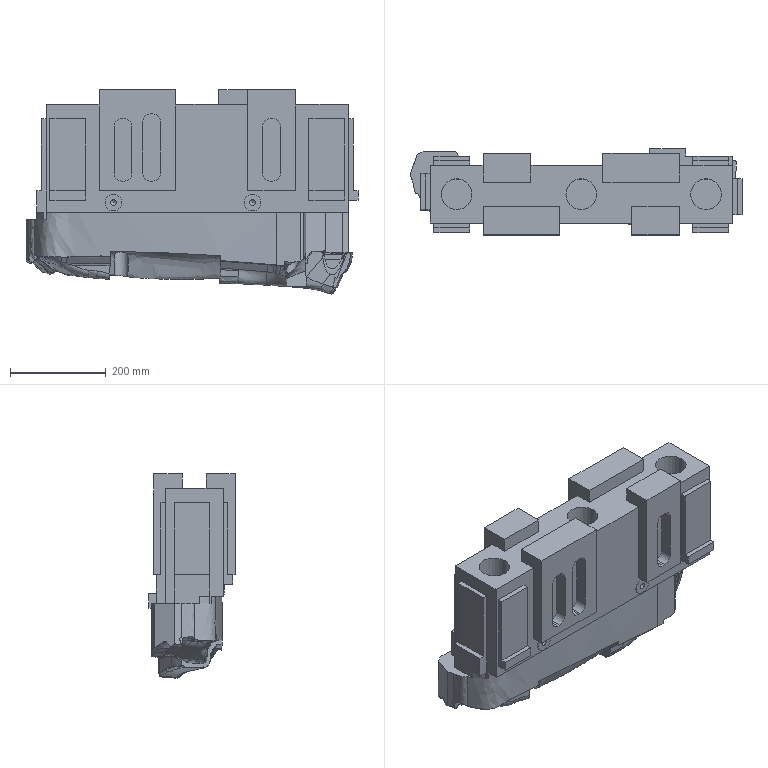Part | NX | features solid 2 | 1 solid | 395 faces | box 692.554 x 180 x 425.876 mm | volume 27420201 mm3 | spline 212 | plane 138 | cylinder 39 | cone 6 | commonest cylinder face diameters 32 x24 12 x6 35 x4 64 x3 30 x2